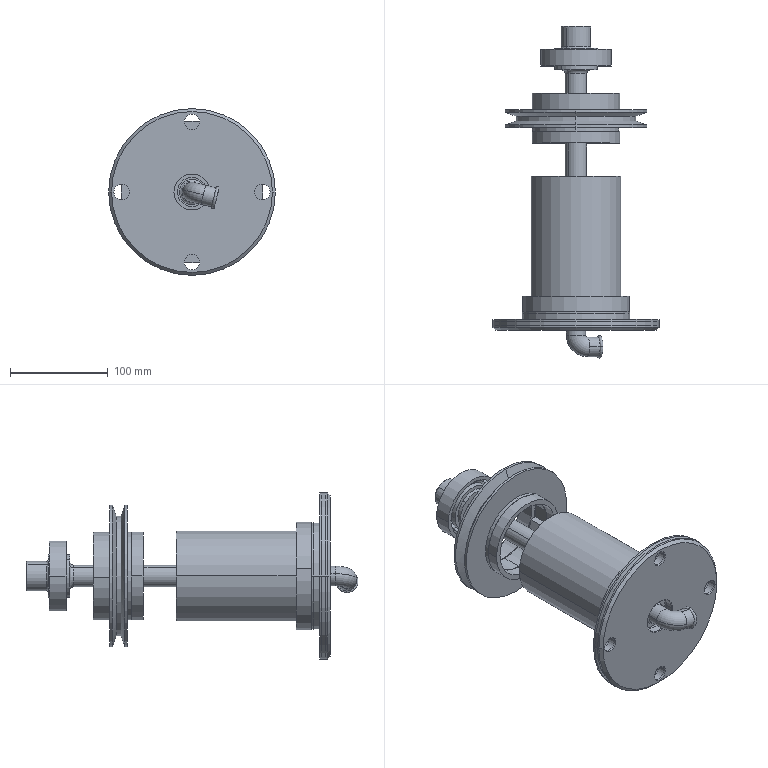Part | NX | features BREP 64 | 89 solids | 574 faces | box 171 x 340.5 x 171 mm | volume 1447890 mm3 | sphere 292 | cylinder 152 | plane 62 | torus 42 | cone 26 | commonest cylinder face diameters 16 x24 3 x16 80 x13 44 x12 22 x8 30 x8